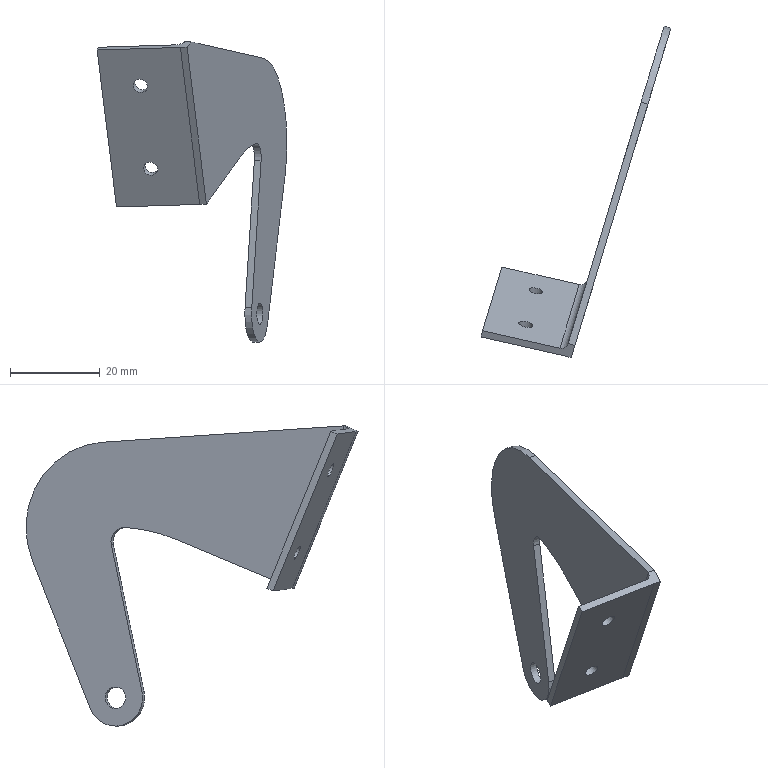Part | NX | features NG well(right door) 2 | 1 solid | 21 faces | box 42.37 x 74.162 x 67.071 mm | volume 4862 mm3 | plane 13 | cylinder 8 | commonest cylinder face diameters 3.175 x2 3.15 x1 4.763 x1 6.35 x1 12.7 x1 38.1 x1
STEP:
#1=CARTESIAN_POINT('',(564.181,-448.408,-122.365));
#2=VERTEX_POINT('',#1);
#3=CARTESIAN_POINT('',(563.493,-450.688,-122.365));
#4=DIRECTION('',(-0.9572,0.2893,0.));
#5=DIRECTION('',(0.2893,0.9572,0.));
#6=AXIS2_PLACEMENT_3D('',#3,#4,#5);
#7=CIRCLE('',#6,2.381);
#8=EDGE_CURVE('',#2,#2,#7,.T.);
#9=ORIENTED_EDGE('',*,*,#8,.F.);
#10=EDGE_LOOP('',(#9));
#11=FACE_BOUND('',#10,.T.);
#12=CARTESIAN_POINT('',(548.065,-501.739,-61.698));
#13=VERTEX_POINT('',#12);
#14=CARTESIAN_POINT('',(548.102,-501.617,-61.644));
#15=VERTEX_POINT('',#14);
#16=CARTESIAN_POINT('',(548.102,-501.617,-61.644));
#17=DIRECTION('',(0.2662,0.8808,0.3916));
#18=VECTOR('',#17,1000.);
#19=LINE('',#16,#18);
#20=EDGE_CURVE('',#13,#15,#19,.T.);
#21=ORIENTED_EDGE('',*,*,#20,.T.);
#22=CARTESIAN_POINT('',(564.377,-447.761,-65.299));
#23=VERTEX_POINT('',#22);
#24=CARTESIAN_POINT('',(548.102,-501.617,-61.644));
#25=DIRECTION('',(0.2887,0.9552,-0.06482));
#26=VECTOR('',#25,1000.);
#27=LINE('',#24,#26);
#28=EDGE_CURVE('',#15,#23,#27,.T.);
#29=ORIENTED_EDGE('',*,*,#28,.T.);
#30=CARTESIAN_POINT('',(569.121,-432.061,-91.511));
#31=VERTEX_POINT('',#30);
#32=CARTESIAN_POINT('',(564.02,-448.943,-84.309));
#33=DIRECTION('',(-0.9572,0.2893,0.));
#34=DIRECTION('',(0.2893,0.9572,0.));
#35=AXIS2_PLACEMENT_3D('',#32,#33,#34);
#36=CIRCLE('',#35,19.05);
#37=EDGE_CURVE('',#23,#31,#36,.T.);
#38=ORIENTED_EDGE('',*,*,#37,.T.);
#39=CARTESIAN_POINT('',(565.193,-445.06,-124.766));
#40=VERTEX_POINT('',#39);
#41=CARTESIAN_POINT('',(565.193,-445.06,-124.766));
#42=DIRECTION('',(-0.1094,-0.3619,-0.9258));
#43=VECTOR('',#42,1000.);
#44=LINE('',#41,#43);
#45=EDGE_CURVE('',#31,#40,#44,.T.);
#46=ORIENTED_EDGE('',*,*,#45,.T.);
#47=CARTESIAN_POINT('',(561.698,-456.626,-121.008));
#48=VERTEX_POINT('',#47);
#49=CARTESIAN_POINT('',(563.493,-450.688,-122.365));
#50=DIRECTION('',(-0.9572,0.2893,0.));
#51=DIRECTION('',(0.2893,0.9572,0.));
#52=AXIS2_PLACEMENT_3D('',#49,#50,#51);
#53=CIRCLE('',#52,6.35);
#54=EDGE_CURVE('',#40,#48,#53,.T.);
#55=ORIENTED_EDGE('',*,*,#54,.T.);
#56=CARTESIAN_POINT('',(563.775,-449.754,-88.183));
#57=VERTEX_POINT('',#56);
#58=CARTESIAN_POINT('',(561.698,-456.626,-121.008));
#59=DIRECTION('',(0.0618,0.2045,0.9769));
#60=VECTOR('',#59,1000.);
#61=LINE('',#58,#60);
#62=EDGE_CURVE('',#48,#57,#61,.T.);
#63=ORIENTED_EDGE('',*,*,#62,.T.);
#64=CARTESIAN_POINT('',(562.822,-452.908,-84.336));
#65=VERTEX_POINT('',#64);
#66=CARTESIAN_POINT('',(562.877,-452.723,-87.505));
#67=DIRECTION('',(-0.9572,0.2893,0.));
#68=DIRECTION('',(0.2893,0.9572,0.));
#69=AXIS2_PLACEMENT_3D('',#66,#67,#68);
#70=CIRCLE('',#69,3.175);
#71=EDGE_CURVE('',#65,#57,#70,.T.);
#72=ORIENTED_EDGE('',*,*,#71,.F.);
#73=CARTESIAN_POINT('',(559.378,-464.303,-87.019));
#74=VERTEX_POINT('',#73);
#75=CARTESIAN_POINT('',(563.493,-450.688,-122.365));
#76=DIRECTION('',(0.9572,-0.2893,0.));
#77=DIRECTION('',(0.2893,0.9572,0.));
#78=AXIS2_PLACEMENT_3D('',#75,#76,#77);
#79=CIRCLE('',#78,38.1);
#80=EDGE_CURVE('',#65,#74,#79,.T.);
#81=ORIENTED_EDGE('',*,*,#80,.T.);
#82=CARTESIAN_POINT('',(552.417,-487.337,-96.702));
#83=VERTEX_POINT('',#82);
#84=CARTESIAN_POINT('',(552.417,-487.337,-96.702));
#85=DIRECTION('',(-0.2684,-0.888,-0.3733));
#86=VECTOR('',#85,1000.);
#87=LINE('',#84,#86);
#88=EDGE_CURVE('',#74,#83,#87,.T.);
#89=ORIENTED_EDGE('',*,*,#88,.T.);
#90=CARTESIAN_POINT('',(552.381,-487.458,-96.756));
#91=VERTEX_POINT('',#90);
#92=CARTESIAN_POINT('',(551.572,-490.134,-97.945));
#93=DIRECTION('',(-0.2662,-0.8808,-0.3916));
#94=VECTOR('',#93,1000.);
#95=LINE('',#92,#94);
#96=EDGE_CURVE('',#83,#91,#95,.T.);
#97=ORIENTED_EDGE('',*,*,#96,.T.);
#98=CARTESIAN_POINT('',(552.381,-487.458,-96.756));
#99=DIRECTION('',(-0.1133,-0.3748,0.9202));
#100=VECTOR('',#99,1000.);
#101=LINE('',#98,#100);
#102=EDGE_CURVE('',#13,#91,#101,.F.);
#103=ORIENTED_EDGE('',*,*,#102,.F.);
#104=EDGE_LOOP('',(#21,#29,#38,#46,#55,#63,#72,#81,#89,#97,#103));
#105=FACE_BOUND('',#104,.T.);
#106=CARTESIAN_POINT('',(563.493,-450.688,-122.365));
#107=DIRECTION('',(0.9572,-0.2893,0.));
#108=DIRECTION('',(0.2893,0.9572,0.));
#109=AXIS2_PLACEMENT_3D('',#106,#107,#108);
#110=PLANE('',#109);
#111=ADVANCED_FACE('',(#11,#105),#110,.F.);
#112=ORIENTED_EDGE('',*,*,#96,.F.);
#113=CARTESIAN_POINT('',(553.925,-487.793,-96.702));
#114=VERTEX_POINT('',#113);
#115=CARTESIAN_POINT('',(552.417,-487.337,-96.702));
#116=DIRECTION('',(0.9572,-0.2893,0.));
#117=VECTOR('',#116,1000.);
#118=LINE('',#115,#117);
#119=EDGE_CURVE('',#83,#114,#118,.T.);
#120=ORIENTED_EDGE('',*,*,#119,.T.);
#121=CARTESIAN_POINT('',(553.08,-490.589,-97.945));
#122=VERTEX_POINT('',#121);
#123=CARTESIAN_POINT('',(553.08,-490.589,-97.945));
#124=DIRECTION('',(-0.2662,-0.8808,-0.3916));
#125=VECTOR('',#124,1000.);
#126=LINE('',#123,#125);
#127=EDGE_CURVE('',#114,#122,#126,.T.);
#128=ORIENTED_EDGE('',*,*,#127,.T.);
#129=CARTESIAN_POINT('',(551.572,-490.134,-97.945));
#130=VERTEX_POINT('',#129);
#131=CARTESIAN_POINT('',(551.572,-490.134,-97.945));
#132=DIRECTION('',(0.9572,-0.2893,0.));
#133=VECTOR('',#132,1000.);
#134=LINE('',#131,#133);
#135=EDGE_CURVE('',#130,#122,#134,.T.);
#136=ORIENTED_EDGE('',*,*,#135,.F.);
#137=CARTESIAN_POINT('',(551.572,-490.134,-97.945));
#138=DIRECTION('',(-0.2662,-0.8808,-0.3916));
#139=VECTOR('',#138,1000.);
#140=LINE('',#137,#139);
#141=EDGE_CURVE('',#91,#130,#140,.T.);
#142=ORIENTED_EDGE('',*,*,#141,.F.);
#143=EDGE_LOOP('',(#112,#120,#128,#136,#142));
#144=FACE_BOUND('',#143,.T.);
#145=CARTESIAN_POINT('',(551.572,-490.134,-97.945));
#146=DIRECTION('',(0.1133,0.3748,-0.9202));
#147=DIRECTION('',(0.,-0.9261,-0.3772));
#148=AXIS2_PLACEMENT_3D('',#145,#146,#147);
#149=PLANE('',#148);
#150=ADVANCED_FACE('',(#144),#149,.T.);
#151=CARTESIAN_POINT('',(560.886,-464.758,-87.019));
#152=VERTEX_POINT('',#151);
#153=CARTESIAN_POINT('',(553.925,-487.793,-96.702));
#154=DIRECTION('',(-0.2684,-0.888,-0.3733));
#155=VECTOR('',#154,1000.);
#156=LINE('',#153,#155);
#157=EDGE_CURVE('',#152,#114,#156,.T.);
#158=ORIENTED_EDGE('',*,*,#157,.T.);
#159=ORIENTED_EDGE('',*,*,#119,.F.);
#160=ORIENTED_EDGE('',*,*,#88,.F.);
#161=CARTESIAN_POINT('',(559.378,-464.303,-87.019));
#162=DIRECTION('',(0.9572,-0.2893,0.));
#163=VECTOR('',#162,1000.);
#164=LINE('',#161,#163);
#165=EDGE_CURVE('',#74,#152,#164,.T.);
#166=ORIENTED_EDGE('',*,*,#165,.T.);
#167=EDGE_LOOP('',(#158,#159,#160,#166));
#168=FACE_BOUND('',#167,.T.);
#169=CARTESIAN_POINT('',(552.417,-487.337,-96.702));
#170=DIRECTION('',(0.108,0.3573,-0.9277));
#171=DIRECTION('',(0.,-0.9332,-0.3594));
#172=AXIS2_PLACEMENT_3D('',#169,#170,#171);
#173=PLANE('',#172);
#174=ADVANCED_FACE('',(#168),#173,.T.);
#175=CARTESIAN_POINT('',(564.329,-453.364,-84.336));
#176=VERTEX_POINT('',#175);
#177=CARTESIAN_POINT('',(565.,-451.143,-122.365));
#178=DIRECTION('',(0.9572,-0.2893,0.));
#179=DIRECTION('',(0.2893,0.9572,0.));
#180=AXIS2_PLACEMENT_3D('',#177,#178,#179);
#181=CIRCLE('',#180,38.1);
#182=EDGE_CURVE('',#176,#152,#181,.T.);
#183=ORIENTED_EDGE('',*,*,#182,.T.);
#184=ORIENTED_EDGE('',*,*,#165,.F.);
#185=ORIENTED_EDGE('',*,*,#80,.F.);
#186=CARTESIAN_POINT('',(562.822,-452.908,-84.336));
#187=DIRECTION('',(0.9572,-0.2893,0.));
#188=VECTOR('',#187,1000.);
#189=LINE('',#186,#188);
#190=EDGE_CURVE('',#176,#65,#189,.F.);
#191=ORIENTED_EDGE('',*,*,#190,.F.);
#192=EDGE_LOOP('',(#183,#184,#185,#191));
#193=FACE_BOUND('',#192,.T.);
#194=CARTESIAN_POINT('',(563.493,-450.688,-122.365));
#195=DIRECTION('',(0.9572,-0.2893,0.));
#196=DIRECTION('',(0.2893,0.9572,0.));
#197=AXIS2_PLACEMENT_3D('',#194,#195,#196);
#198=CYLINDRICAL_SURFACE('',#197,38.1);
#199=ADVANCED_FACE('',(#193),#198,.F.);
#200=ORIENTED_EDGE('',*,*,#62,.F.);
#201=CARTESIAN_POINT('',(563.206,-457.082,-121.008));
#202=VERTEX_POINT('',#201);
#203=CARTESIAN_POINT('',(561.698,-456.626,-121.008));
#204=DIRECTION('',(0.9572,-0.2893,0.));
#205=VECTOR('',#204,1000.);
#206=LINE('',#203,#205);
#207=EDGE_CURVE('',#48,#202,#206,.T.);
#208=ORIENTED_EDGE('',*,*,#207,.T.);
#209=CARTESIAN_POINT('',(565.282,-450.21,-88.183));
#210=VERTEX_POINT('',#209);
#211=CARTESIAN_POINT('',(563.206,-457.082,-121.008));
#212=DIRECTION('',(0.0618,0.2045,0.9769));
#213=VECTOR('',#212,1000.);
#214=LINE('',#211,#213);
#215=EDGE_CURVE('',#202,#210,#214,.T.);
#216=ORIENTED_EDGE('',*,*,#215,.T.);
#217=CARTESIAN_POINT('',(565.282,-450.21,-88.183));
#218=DIRECTION('',(-0.9572,0.2893,0.));
#219=VECTOR('',#218,1000.);
#220=LINE('',#217,#219);
#221=EDGE_CURVE('',#57,#210,#220,.F.);
#222=ORIENTED_EDGE('',*,*,#221,.F.);
#223=EDGE_LOOP('',(#200,#208,#216,#222));
#224=FACE_BOUND('',#223,.T.);
#225=CARTESIAN_POINT('',(561.698,-456.626,-121.008));
#226=DIRECTION('',(-0.2826,-0.9351,0.2136));
#227=DIRECTION('',(0.9572,-0.2893,0.));
#228=AXIS2_PLACEMENT_3D('',#225,#226,#227);
#229=PLANE('',#228);
#230=ADVANCED_FACE('',(#224),#229,.T.);
#231=CARTESIAN_POINT('',(566.701,-445.516,-124.766));
#232=VERTEX_POINT('',#231);
#233=CARTESIAN_POINT('',(565.,-451.143,-122.365));
#234=DIRECTION('',(-0.9572,0.2893,0.));
#235=DIRECTION('',(0.2893,0.9572,0.));
#236=AXIS2_PLACEMENT_3D('',#233,#234,#235);
#237=CIRCLE('',#236,6.35);
#238=EDGE_CURVE('',#232,#202,#237,.T.);
#239=ORIENTED_EDGE('',*,*,#238,.T.);
#240=ORIENTED_EDGE('',*,*,#207,.F.);
#241=ORIENTED_EDGE('',*,*,#54,.F.);
#242=CARTESIAN_POINT('',(565.193,-445.06,-124.766));
#243=DIRECTION('',(0.9572,-0.2893,0.));
#244=VECTOR('',#243,1000.);
#245=LINE('',#242,#244);
#246=EDGE_CURVE('',#40,#232,#245,.T.);
#247=ORIENTED_EDGE('',*,*,#246,.T.);
#248=EDGE_LOOP('',(#239,#240,#241,#247));
#249=FACE_BOUND('',#248,.T.);
#250=CARTESIAN_POINT('',(563.493,-450.688,-122.365));
#251=DIRECTION('',(0.9572,-0.2893,0.));
#252=DIRECTION('',(0.2893,0.9572,0.));
#253=AXIS2_PLACEMENT_3D('',#250,#251,#252);
#254=CYLINDRICAL_SURFACE('',#253,6.35);
#255=ADVANCED_FACE('',(#249),#254,.T.);
#256=CARTESIAN_POINT('',(570.629,-432.516,-91.511));
#257=VERTEX_POINT('',#256);
#258=CARTESIAN_POINT('',(566.701,-445.516,-124.766));
#259=DIRECTION('',(-0.1094,-0.3619,-0.9258));
#260=VECTOR('',#259,1000.);
#261=LINE('',#258,#260);
#262=EDGE_CURVE('',#257,#232,#261,.T.);
#263=ORIENTED_EDGE('',*,*,#262,.T.);
#264=ORIENTED_EDGE('',*,*,#246,.F.);
#265=ORIENTED_EDGE('',*,*,#45,.F.);
#266=CARTESIAN_POINT('',(569.121,-432.061,-91.511));
#267=DIRECTION('',(0.9572,-0.2893,0.));
#268=VECTOR('',#267,1000.);
#269=LINE('',#266,#268);
#270=EDGE_CURVE('',#31,#257,#269,.T.);
#271=ORIENTED_EDGE('',*,*,#270,.T.);
#272=EDGE_LOOP('',(#263,#264,#265,#271));
#273=FACE_BOUND('',#272,.T.);
#274=CARTESIAN_POINT('',(565.193,-445.06,-124.766));
#275=DIRECTION('',(0.2678,0.8862,-0.3781));
#276=DIRECTION('',(0.,-0.3924,-0.9198));
#277=AXIS2_PLACEMENT_3D('',#274,#275,#276);
#278=PLANE('',#277);
#279=ADVANCED_FACE('',(#273),#278,.T.);
#280=CARTESIAN_POINT('',(565.884,-448.217,-65.299));
#281=VERTEX_POINT('',#280);
#282=CARTESIAN_POINT('',(565.527,-449.399,-84.309));
#283=DIRECTION('',(-0.9572,0.2893,0.));
#284=DIRECTION('',(0.2893,0.9572,0.));
#285=AXIS2_PLACEMENT_3D('',#282,#283,#284);
#286=CIRCLE('',#285,19.05);
#287=EDGE_CURVE('',#281,#257,#286,.T.);
#288=ORIENTED_EDGE('',*,*,#287,.T.);
#289=ORIENTED_EDGE('',*,*,#270,.F.);
#290=ORIENTED_EDGE('',*,*,#37,.F.);
#291=CARTESIAN_POINT('',(564.377,-447.761,-65.299));
#292=DIRECTION('',(0.9572,-0.2893,0.));
#293=VECTOR('',#292,1000.);
#294=LINE('',#291,#293);
#295=EDGE_CURVE('',#23,#281,#294,.T.);
#296=ORIENTED_EDGE('',*,*,#295,.T.);
#297=EDGE_LOOP('',(#288,#289,#290,#296));
#298=FACE_BOUND('',#297,.T.);
#299=CARTESIAN_POINT('',(564.02,-448.943,-84.309));
#300=DIRECTION('',(0.9572,-0.2893,0.));
#301=DIRECTION('',(0.2893,0.9572,0.));
#302=AXIS2_PLACEMENT_3D('',#299,#300,#301);
#303=CYLINDRICAL_SURFACE('',#302,19.05);
#304=ADVANCED_FACE('',(#298),#303,.T.);
#305=CARTESIAN_POINT('',(549.609,-502.073,-61.644));
#306=VERTEX_POINT('',#305);
#307=CARTESIAN_POINT('',(549.609,-502.073,-61.644));
#308=DIRECTION('',(0.2887,0.9552,-0.06482));
#309=VECTOR('',#308,1000.);
#310=LINE('',#307,#309);
#311=EDGE_CURVE('',#306,#281,#310,.T.);
#312=ORIENTED_EDGE('',*,*,#311,.T.);
#313=ORIENTED_EDGE('',*,*,#295,.F.);
#314=ORIENTED_EDGE('',*,*,#28,.F.);
#315=CARTESIAN_POINT('',(548.102,-501.617,-61.644));
#316=DIRECTION('',(0.9572,-0.2893,0.));
#317=VECTOR('',#316,1000.);
#318=LINE('',#315,#317);
#319=EDGE_CURVE('',#15,#306,#318,.T.);
#320=ORIENTED_EDGE('',*,*,#319,.T.);
#321=EDGE_LOOP('',(#312,#313,#314,#320));
#322=FACE_BOUND('',#321,.T.);
#323=CARTESIAN_POINT('',(548.102,-501.617,-61.644));
#324=DIRECTION('',(0.01875,0.06205,0.9979));
#325=DIRECTION('',(0.,0.9981,-0.06206));
#326=AXIS2_PLACEMENT_3D('',#323,#324,#325);
#327=PLANE('',#326);
#328=ADVANCED_FACE('',(#322),#327,.T.);
#329=CARTESIAN_POINT('',(546.256,-502.701,-62.313));
#330=VERTEX_POINT('',#329);
#331=CARTESIAN_POINT('',(528.969,-498.792,-62.848));
#332=VERTEX_POINT('',#331);
#333=CARTESIAN_POINT('',(528.969,-498.792,-62.848));
#334=DIRECTION('',(-0.9749,0.2205,-0.0302));
#335=VECTOR('',#334,1000.);
#336=LINE('',#333,#335);
#337=EDGE_CURVE('',#330,#332,#336,.T.);
#338=ORIENTED_EDGE('',*,*,#337,.T.);
#339=CARTESIAN_POINT('',(528.668,-500.21,-63.463));
#340=VERTEX_POINT('',#339);
#341=CARTESIAN_POINT('',(528.969,-498.792,-62.848));
#342=DIRECTION('',(-0.1916,-0.9005,-0.3904));
#343=VECTOR('',#342,1000.);
#344=LINE('',#341,#343);
#345=EDGE_CURVE('',#332,#340,#344,.T.);
#346=ORIENTED_EDGE('',*,*,#345,.T.);
#347=CARTESIAN_POINT('',(547.257,-504.414,-62.887));
#348=VERTEX_POINT('',#347);
#349=CARTESIAN_POINT('',(528.668,-500.21,-63.463));
#350=DIRECTION('',(-0.9749,0.2205,-0.0302));
#351=VECTOR('',#350,1000.);
#352=LINE('',#349,#351);
#353=EDGE_CURVE('',#348,#340,#352,.T.);
#354=ORIENTED_EDGE('',*,*,#353,.F.);
#355=CARTESIAN_POINT('',(548.764,-504.869,-62.887));
#356=VERTEX_POINT('',#355);
#357=CARTESIAN_POINT('',(547.257,-504.414,-62.887));
#358=DIRECTION('',(0.9572,-0.2893,0.));
#359=VECTOR('',#358,1000.);
#360=LINE('',#357,#359);
#361=EDGE_CURVE('',#348,#356,#360,.T.);
#362=ORIENTED_EDGE('',*,*,#361,.T.);
#363=CARTESIAN_POINT('',(549.609,-502.073,-61.644));
#364=DIRECTION('',(0.2662,0.8808,0.3916));
#365=VECTOR('',#364,1000.);
#366=LINE('',#363,#365);
#367=EDGE_CURVE('',#356,#306,#366,.T.);
#368=ORIENTED_EDGE('',*,*,#367,.T.);
#369=ORIENTED_EDGE('',*,*,#319,.F.);
#370=ORIENTED_EDGE('',*,*,#20,.F.);
#371=CARTESIAN_POINT('',(546.558,-501.283,-61.698));
#372=DIRECTION('',(0.1133,0.3748,-0.9202));
#373=DIRECTION('',(0.,0.9261,0.3772));
#374=AXIS2_PLACEMENT_3D('',#371,#372,#373);
#375=CIRCLE('',#374,1.575);
#376=EDGE_CURVE('',#330,#13,#375,.F.);
#377=ORIENTED_EDGE('',*,*,#376,.F.);
#378=EDGE_LOOP('',(#338,#346,#354,#362,#368,#369,#370,#377));
#379=FACE_BOUND('',#378,.T.);
#380=CARTESIAN_POINT('',(548.102,-501.617,-61.644));
#381=DIRECTION('',(-0.1133,-0.3748,0.9202));
#382=DIRECTION('',(0.,0.9261,0.3772));
#383=AXIS2_PLACEMENT_3D('',#380,#381,#382);
#384=PLANE('',#383);
#385=ADVANCED_FACE('',(#379),#384,.T.);
#386=CARTESIAN_POINT('',(553.08,-490.589,-97.945));
#387=DIRECTION('',(-0.1133,-0.3748,0.9202));
#388=VECTOR('',#387,1000.);
#389=LINE('',#386,#388);
#390=EDGE_CURVE('',#122,#356,#389,.T.);
#391=ORIENTED_EDGE('',*,*,#390,.T.);
#392=ORIENTED_EDGE('',*,*,#361,.F.);
#393=CARTESIAN_POINT('',(551.572,-490.134,-97.945));
#394=DIRECTION('',(-0.1133,-0.3748,0.9202));
#395=VECTOR('',#394,1000.);
#396=LINE('',#393,#395);
#397=EDGE_CURVE('',#130,#348,#396,.T.);
#398=ORIENTED_EDGE('',*,*,#397,.F.);
#399=ORIENTED_EDGE('',*,*,#135,.T.);
#400=EDGE_LOOP('',(#391,#392,#398,#399));
#401=FACE_BOUND('',#400,.T.);
#402=CARTESIAN_POINT('',(551.572,-490.134,-97.945));
#403=DIRECTION('',(-0.2662,-0.8808,-0.3916));
#404=DIRECTION('',(0.,-0.4062,0.9138));
#405=AXIS2_PLACEMENT_3D('',#402,#403,#404);
#406=PLANE('',#405);
#407=ADVANCED_FACE('',(#401),#406,.T.);
#408=CARTESIAN_POINT('',(565.689,-448.864,-122.365));
#409=VERTEX_POINT('',#408);
#410=CARTESIAN_POINT('',(565.,-451.143,-122.365));
#411=DIRECTION('',(-0.9572,0.2893,0.));
#412=DIRECTION('',(0.2893,0.9572,0.));
#413=AXIS2_PLACEMENT_3D('',#410,#411,#412);
#414=CIRCLE('',#413,2.381);
#415=EDGE_CURVE('',#409,#409,#414,.T.);
#416=ORIENTED_EDGE('',*,*,#415,.T.);
#417=EDGE_LOOP('',(#416));
#418=FACE_BOUND('',#417,.T.);
#419=ORIENTED_EDGE('',*,*,#127,.F.);
#420=ORIENTED_EDGE('',*,*,#157,.F.);
#421=ORIENTED_EDGE('',*,*,#182,.F.);
#422=CARTESIAN_POINT('',(564.385,-453.179,-87.505));
#423=DIRECTION('',(-0.9572,0.2893,0.));
#424=DIRECTION('',(0.2893,0.9572,0.));
#425=AXIS2_PLACEMENT_3D('',#422,#423,#424);
#426=CIRCLE('',#425,3.175);
#427=EDGE_CURVE('',#210,#176,#426,.F.);
#428=ORIENTED_EDGE('',*,*,#427,.F.);
#429=ORIENTED_EDGE('',*,*,#215,.F.);
#430=ORIENTED_EDGE('',*,*,#238,.F.);
#431=ORIENTED_EDGE('',*,*,#262,.F.);
#432=ORIENTED_EDGE('',*,*,#287,.F.);
#433=ORIENTED_EDGE('',*,*,#311,.F.);
#434=ORIENTED_EDGE('',*,*,#367,.F.);
#435=ORIENTED_EDGE('',*,*,#390,.F.);
#436=EDGE_LOOP('',(#419,#420,#421,#428,#429,#430,#431,#432,#433,#434,#435));
#437=FACE_BOUND('',#436,.T.);
#438=CARTESIAN_POINT('',(565.,-451.143,-122.365));
#439=DIRECTION('',(0.9572,-0.2893,0.));
#440=DIRECTION('',(0.2893,0.9572,0.));
#441=AXIS2_PLACEMENT_3D('',#438,#439,#440);
#442=PLANE('',#441);
#443=ADVANCED_FACE('',(#418,#437),#442,.T.);
#444=ORIENTED_EDGE('',*,*,#8,.T.);
#445=EDGE_LOOP('',(#444));
#446=FACE_BOUND('',#445,.T.);
#447=ORIENTED_EDGE('',*,*,#415,.F.);
#448=EDGE_LOOP('',(#447));
#449=FACE_BOUND('',#448,.T.);
#450=CARTESIAN_POINT('',(563.493,-450.688,-122.365));
#451=DIRECTION('',(0.9572,-0.2893,0.));
#452=DIRECTION('',(0.2893,0.9572,0.));
#453=AXIS2_PLACEMENT_3D('',#450,#451,#452);
#454=CYLINDRICAL_SURFACE('',#453,2.381);
#455=ADVANCED_FACE('',(#446,#449),#454,.F.);
#456=ORIENTED_EDGE('',*,*,#71,.T.);
#457=ORIENTED_EDGE('',*,*,#221,.T.);
#458=ORIENTED_EDGE('',*,*,#427,.T.);
#459=ORIENTED_EDGE('',*,*,#190,.T.);
#460=EDGE_LOOP('',(#456,#457,#458,#459));
#461=FACE_BOUND('',#460,.T.);
#462=CARTESIAN_POINT('',(562.877,-452.723,-87.505));
#463=DIRECTION('',(0.9572,-0.2893,0.));
#464=DIRECTION('',(0.2893,0.9572,0.));
#465=AXIS2_PLACEMENT_3D('',#462,#463,#464);
#466=CYLINDRICAL_SURFACE('',#465,3.175);
#467=ADVANCED_FACE('',(#461),#466,.F.);
#468=CARTESIAN_POINT('',(532.983,-485.93,-98.521));
#469=VERTEX_POINT('',#468);
#470=CARTESIAN_POINT('',(553.103,-490.48,-97.898));
#471=DIRECTION('',(0.9749,-0.2205,0.0302));
#472=VECTOR('',#471,1000.);
#473=LINE('',#470,#472);
#474=EDGE_CURVE('',#469,#130,#473,.T.);
#475=ORIENTED_EDGE('',*,*,#474,.F.);
#476=CARTESIAN_POINT('',(533.285,-484.512,-97.906));
#477=VERTEX_POINT('',#476);
#478=CARTESIAN_POINT('',(533.285,-484.512,-97.906));
#479=DIRECTION('',(-0.1916,-0.9005,-0.3904));
#480=VECTOR('',#479,1000.);
#481=LINE('',#478,#480);
#482=EDGE_CURVE('',#477,#469,#481,.T.);
#483=ORIENTED_EDGE('',*,*,#482,.F.);
#484=CARTESIAN_POINT('',(550.572,-488.421,-97.371));
#485=VERTEX_POINT('',#484);
#486=CARTESIAN_POINT('',(553.405,-489.062,-97.283));
#487=DIRECTION('',(0.9749,-0.2205,0.0302));
#488=VECTOR('',#487,1000.);
#489=LINE('',#486,#488);
#490=EDGE_CURVE('',#477,#485,#489,.T.);
#491=ORIENTED_EDGE('',*,*,#490,.T.);
#492=CARTESIAN_POINT('',(550.873,-487.003,-96.756));
#493=DIRECTION('',(0.1133,0.3748,-0.9202));
#494=DIRECTION('',(0.,0.9261,0.3772));
#495=AXIS2_PLACEMENT_3D('',#492,#493,#494);
#496=CIRCLE('',#495,1.575);
#497=EDGE_CURVE('',#91,#485,#496,.T.);
#498=ORIENTED_EDGE('',*,*,#497,.F.);
#499=ORIENTED_EDGE('',*,*,#141,.T.);
#500=EDGE_LOOP('',(#475,#483,#491,#498,#499));
#501=FACE_BOUND('',#500,.T.);
#502=CARTESIAN_POINT('',(553.405,-489.062,-97.283));
#503=DIRECTION('',(-0.1133,-0.3748,0.9202));
#504=DIRECTION('',(0.,0.9261,0.3772));
#505=AXIS2_PLACEMENT_3D('',#502,#503,#504);
#506=PLANE('',#505);
#507=ADVANCED_FACE('',(#501),#506,.F.);
#508=CARTESIAN_POINT('',(538.632,-496.742,-72.319));
#509=VERTEX_POINT('',#508);
#510=CARTESIAN_POINT('',(538.632,-497.373,-70.862));
#511=DIRECTION('',(-0.1916,-0.9005,-0.3904));
#512=DIRECTION('',(0.,0.3978,-0.9175));
#513=AXIS2_PLACEMENT_3D('',#510,#511,#512);
#514=CIRCLE('',#513,1.587);
#515=EDGE_CURVE('',#509,#509,#514,.T.);
#516=ORIENTED_EDGE('',*,*,#515,.T.);
#517=EDGE_LOOP('',(#516));
#518=FACE_BOUND('',#517,.T.);
#519=CARTESIAN_POINT('',(540.909,-489.208,-90.814));
#520=VERTEX_POINT('',#519);
#521=CARTESIAN_POINT('',(540.909,-489.84,-89.357));
#522=DIRECTION('',(-0.1916,-0.9005,-0.3904));
#523=DIRECTION('',(0.,0.3978,-0.9175));
#524=AXIS2_PLACEMENT_3D('',#521,#522,#523);
#525=CIRCLE('',#524,1.587);
#526=EDGE_CURVE('',#520,#520,#525,.T.);
#527=ORIENTED_EDGE('',*,*,#526,.T.);
#528=EDGE_LOOP('',(#527));
#529=FACE_BOUND('',#528,.T.);
#530=ORIENTED_EDGE('',*,*,#490,.F.);
#531=CARTESIAN_POINT('',(533.285,-484.512,-97.906));
#532=DIRECTION('',(0.1133,0.3748,-0.9202));
#533=VECTOR('',#532,1000.);
#534=LINE('',#531,#533);
#535=EDGE_CURVE('',#332,#477,#534,.T.);
#536=ORIENTED_EDGE('',*,*,#535,.F.);
#537=ORIENTED_EDGE('',*,*,#337,.F.);
#538=CARTESIAN_POINT('',(546.256,-502.701,-62.313));
#539=DIRECTION('',(-0.1133,-0.3748,0.9202));
#540=VECTOR('',#539,1000.);
#541=LINE('',#538,#540);
#542=EDGE_CURVE('',#485,#330,#541,.T.);
#543=ORIENTED_EDGE('',*,*,#542,.F.);
#544=EDGE_LOOP('',(#530,#536,#537,#543));
#545=FACE_BOUND('',#544,.T.);
#546=CARTESIAN_POINT('',(549.089,-503.342,-62.225));
#547=DIRECTION('',(-0.1916,-0.9005,-0.3904));
#548=DIRECTION('',(0.,-0.3978,0.9175));
#549=AXIS2_PLACEMENT_3D('',#546,#547,#548);
#550=PLANE('',#549);
#551=ADVANCED_FACE('',(#518,#529,#545),#550,.F.);
#552=CARTESIAN_POINT('',(538.33,-498.16,-72.933));
#553=VERTEX_POINT('',#552);
#554=CARTESIAN_POINT('',(538.33,-498.791,-71.477));
#555=DIRECTION('',(-0.1916,-0.9005,-0.3904));
#556=DIRECTION('',(0.,0.3978,-0.9175));
#557=AXIS2_PLACEMENT_3D('',#554,#555,#556);
#558=CIRCLE('',#557,1.587);
#559=EDGE_CURVE('',#553,#553,#558,.T.);
#560=ORIENTED_EDGE('',*,*,#559,.F.);
#561=EDGE_LOOP('',(#560));
#562=FACE_BOUND('',#561,.T.);
#563=CARTESIAN_POINT('',(540.607,-490.626,-91.429));
#564=VERTEX_POINT('',#563);
#565=CARTESIAN_POINT('',(540.607,-491.258,-89.972));
#566=DIRECTION('',(-0.1916,-0.9005,-0.3904));
#567=DIRECTION('',(0.,0.3978,-0.9175));
#568=AXIS2_PLACEMENT_3D('',#565,#566,#567);
#569=CIRCLE('',#568,1.587);
#570=EDGE_CURVE('',#564,#564,#569,.T.);
#571=ORIENTED_EDGE('',*,*,#570,.F.);
#572=EDGE_LOOP('',(#571));
#573=FACE_BOUND('',#572,.T.);
#574=ORIENTED_EDGE('',*,*,#397,.T.);
#575=ORIENTED_EDGE('',*,*,#353,.T.);
#576=CARTESIAN_POINT('',(532.983,-485.93,-98.521));
#577=DIRECTION('',(0.1133,0.3748,-0.9202));
#578=VECTOR('',#577,1000.);
#579=LINE('',#576,#578);
#580=EDGE_CURVE('',#340,#469,#579,.T.);
#581=ORIENTED_EDGE('',*,*,#580,.T.);
#582=ORIENTED_EDGE('',*,*,#474,.T.);
#583=EDGE_LOOP('',(#574,#575,#581,#582));
#584=FACE_BOUND('',#583,.T.);
#585=CARTESIAN_POINT('',(548.788,-504.76,-62.84));
#586=DIRECTION('',(-0.1916,-0.9005,-0.3904));
#587=DIRECTION('',(0.,-0.3978,0.9175));
#588=AXIS2_PLACEMENT_3D('',#585,#586,#587);
#589=PLANE('',#588);
#590=ADVANCED_FACE('',(#562,#573,#584),#589,.T.);
#591=ORIENTED_EDGE('',*,*,#580,.F.);
#592=ORIENTED_EDGE('',*,*,#345,.F.);
#593=ORIENTED_EDGE('',*,*,#535,.T.);
#594=ORIENTED_EDGE('',*,*,#482,.T.);
#595=EDGE_LOOP('',(#591,#592,#593,#594));
#596=FACE_BOUND('',#595,.T.);
#597=CARTESIAN_POINT('',(533.285,-484.512,-97.906));
#598=DIRECTION('',(0.9749,-0.2205,0.0302));
#599=DIRECTION('',(0.2206,0.9754,0.));
#600=AXIS2_PLACEMENT_3D('',#597,#598,#599);
#601=PLANE('',#600);
#602=ADVANCED_FACE('',(#596),#601,.F.);
#603=ORIENTED_EDGE('',*,*,#497,.T.);
#604=ORIENTED_EDGE('',*,*,#542,.T.);
#605=ORIENTED_EDGE('',*,*,#376,.T.);
#606=ORIENTED_EDGE('',*,*,#102,.T.);
#607=EDGE_LOOP('',(#603,#604,#605,#606));
#608=FACE_BOUND('',#607,.T.);
#609=CARTESIAN_POINT('',(546.558,-501.283,-61.698));
#610=DIRECTION('',(0.1133,0.3748,-0.9202));
#611=DIRECTION('',(0.,-0.9261,-0.3772));
#612=AXIS2_PLACEMENT_3D('',#609,#610,#611);
#613=CYLINDRICAL_SURFACE('',#612,1.575);
#614=ADVANCED_FACE('',(#608),#613,.F.);
#615=ORIENTED_EDGE('',*,*,#570,.T.);
#616=EDGE_LOOP('',(#615));
#617=FACE_BOUND('',#616,.T.);
#618=ORIENTED_EDGE('',*,*,#526,.F.);
#619=EDGE_LOOP('',(#618));
#620=FACE_BOUND('',#619,.T.);
#621=CARTESIAN_POINT('',(540.909,-489.84,-89.357));
#622=DIRECTION('',(-0.1916,-0.9005,-0.3904));
#623=DIRECTION('',(0.,0.3978,-0.9175));
#624=AXIS2_PLACEMENT_3D('',#621,#622,#623);
#625=CYLINDRICAL_SURFACE('',#624,1.587);
#626=ADVANCED_FACE('',(#617,#620),#625,.F.);
#627=ORIENTED_EDGE('',*,*,#559,.T.);
#628=EDGE_LOOP('',(#627));
#629=FACE_BOUND('',#628,.T.);
#630=ORIENTED_EDGE('',*,*,#515,.F.);
#631=EDGE_LOOP('',(#630));
#632=FACE_BOUND('',#631,.T.);
#633=CARTESIAN_POINT('',(538.632,-497.373,-70.862));
#634=DIRECTION('',(-0.1916,-0.9005,-0.3904));
#635=DIRECTION('',(0.,0.3978,-0.9175));
#636=AXIS2_PLACEMENT_3D('',#633,#634,#635);
#637=CYLINDRICAL_SURFACE('',#636,1.587);
#638=ADVANCED_FACE('',(#629,#632),#637,.F.);
#639=CLOSED_SHELL('',(#111,#150,#174,#199,#230,#255,#279,#304,#328,#385,#407,#443,#455,#467,#507,#551,#590,#602,#614,#626,#638));
#640=MANIFOLD_SOLID_BREP('',#639);
#641=(LENGTH_UNIT()NAMED_UNIT(*)SI_UNIT(.MILLI.,.METRE.));
#642=UNCERTAINTY_MEASURE_WITH_UNIT(LENGTH_MEASURE(0.00001),#641,'','');
#643=(NAMED_UNIT(*)PLANE_ANGLE_UNIT()SI_UNIT($,.RADIAN.));
#644=(NAMED_UNIT(*)SI_UNIT($,.STERADIAN.)SOLID_ANGLE_UNIT());
#645=(GEOMETRIC_REPRESENTATION_CONTEXT(3)GLOBAL_UNCERTAINTY_ASSIGNED_CONTEXT((#642))GLOBAL_UNIT_ASSIGNED_CONTEXT((#641,#643,#644))REPRESENTATION_CONTEXT('',''));
#646=ADVANCED_BREP_SHAPE_REPRESENTATION('',(#640),#645);